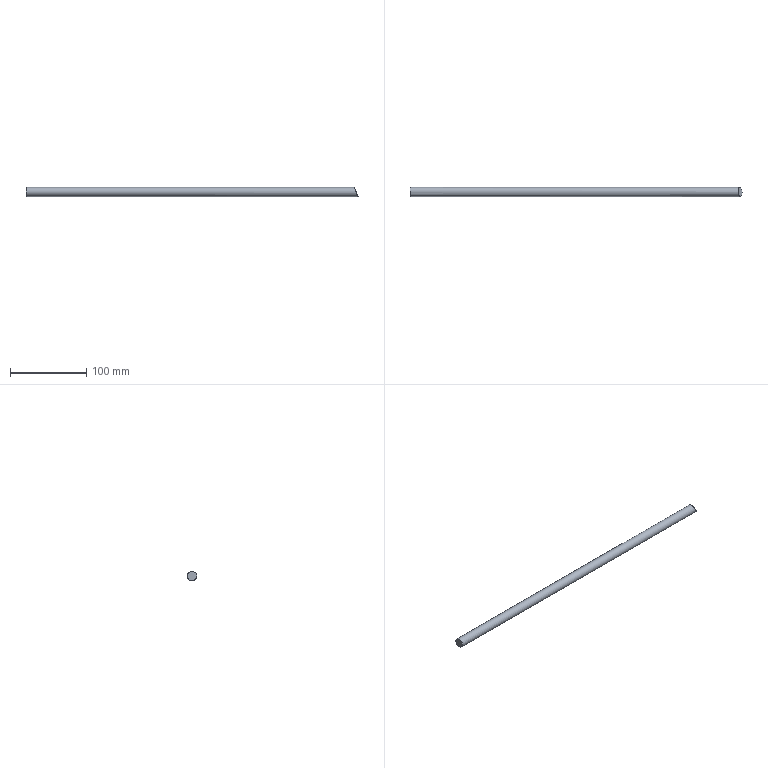Part | STEP file | solid 188 | 1 solid | 3 faces | box 435.109 x 12 x 12 mm | volume 48874 mm3 | cylinder 1 | spline 1 | plane 1 | commonest cylinder face diameters 12 x1